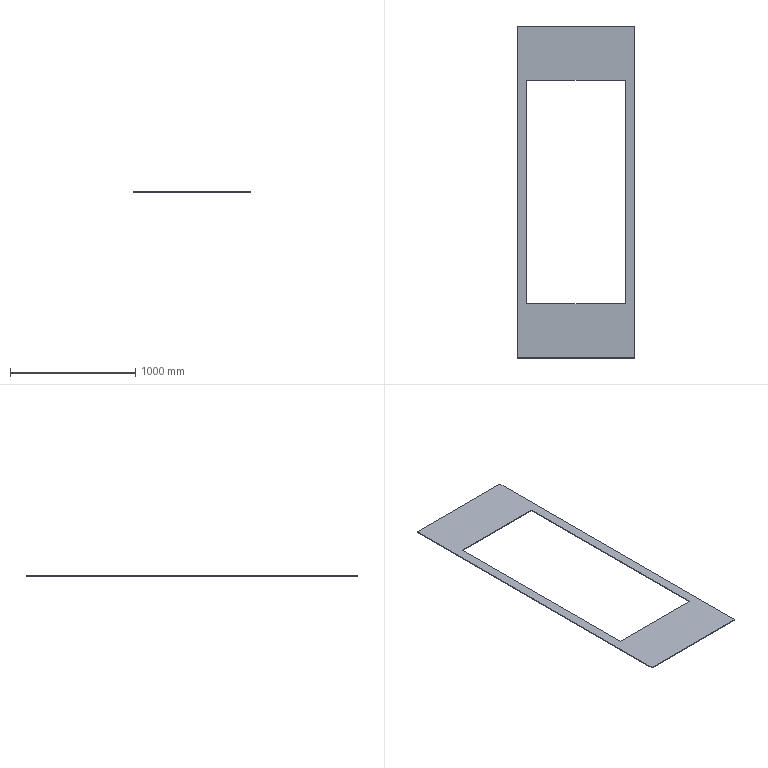Part | STEP file | Bottom plate 6_Default<As machined> | 1 solid | 10 faces | box 934 x 2650 x 6 mm | volume 6458664 mm3 | plane 10
STEP:
#1=CARTESIAN_POINT('',(0.,0.,0.));
#2=DIRECTION('',(0.,0.,1.));
#3=DIRECTION('',(1.,0.,0.));
#4=AXIS2_PLACEMENT_3D('',#1,#2,#3);
#5=CARTESIAN_POINT('',(467.,-1325.,6.));
#6=VERTEX_POINT('',#5);
#7=CARTESIAN_POINT('',(467.,1325.,6.));
#8=VERTEX_POINT('',#7);
#9=CARTESIAN_POINT('',(467.,1325.,6.));
#10=DIRECTION('',(0.,1.,0.));
#11=VECTOR('',#10,1.);
#12=LINE('',#9,#11);
#13=CARTESIAN_POINT('',(0.,0.,6.));
#14=DIRECTION('',(0.,0.,1.));
#15=DIRECTION('',(1.,0.,0.));
#16=AXIS2_PLACEMENT_3D('',#13,#14,#15);
#17=PLANE('',#16);
#18=CARTESIAN_POINT('',(467.,1325.));
#19=DIRECTION('',(0.,1.));
#20=VECTOR('',#19,1.);
#21=LINE('',#18,#20);
#22=(GEOMETRIC_REPRESENTATION_CONTEXT(2)PARAMETRIC_REPRESENTATION_CONTEXT()REPRESENTATION_CONTEXT('',''));
#23=DEFINITIONAL_REPRESENTATION('',(#21),#22);
#24=PCURVE('',#17,#23);
#25=CARTESIAN_POINT('',(467.,1325.,6.));
#26=DIRECTION('',(-1.,0.,0.));
#27=DIRECTION('',(0.,-1.,0.));
#28=AXIS2_PLACEMENT_3D('',#25,#26,#27);
#29=PLANE('',#28);
#30=CARTESIAN_POINT('',(0.,0.));
#31=DIRECTION('',(-1.,0.));
#32=VECTOR('',#31,1.);
#33=LINE('',#30,#32);
#34=(GEOMETRIC_REPRESENTATION_CONTEXT(2)PARAMETRIC_REPRESENTATION_CONTEXT()REPRESENTATION_CONTEXT('',''));
#35=DEFINITIONAL_REPRESENTATION('',(#33),#34);
#36=PCURVE('',#29,#35);
#37=SURFACE_CURVE('',#12,(#24,#36),.PCURVE_S1.);
#38=EDGE_CURVE('',#6,#8,#37,.T.);
#39=ORIENTED_EDGE('',*,*,#38,.T.);
#40=CARTESIAN_POINT('',(-467.,1325.,6.));
#41=VERTEX_POINT('',#40);
#42=CARTESIAN_POINT('',(-467.,1325.,6.));
#43=DIRECTION('',(-1.,0.,0.));
#44=VECTOR('',#43,1.);
#45=LINE('',#42,#44);
#46=CARTESIAN_POINT('',(-467.,1325.));
#47=DIRECTION('',(-1.,0.));
#48=VECTOR('',#47,1.);
#49=LINE('',#46,#48);
#50=(GEOMETRIC_REPRESENTATION_CONTEXT(2)PARAMETRIC_REPRESENTATION_CONTEXT()REPRESENTATION_CONTEXT('',''));
#51=DEFINITIONAL_REPRESENTATION('',(#49),#50);
#52=PCURVE('',#17,#51);
#53=CARTESIAN_POINT('',(-467.,1325.,6.));
#54=DIRECTION('',(0.,-1.,0.));
#55=DIRECTION('',(0.,0.,-1.));
#56=AXIS2_PLACEMENT_3D('',#53,#54,#55);
#57=PLANE('',#56);
#58=CARTESIAN_POINT('',(0.,0.));
#59=DIRECTION('',(0.,-1.));
#60=VECTOR('',#59,1.);
#61=LINE('',#58,#60);
#62=(GEOMETRIC_REPRESENTATION_CONTEXT(2)PARAMETRIC_REPRESENTATION_CONTEXT()REPRESENTATION_CONTEXT('',''));
#63=DEFINITIONAL_REPRESENTATION('',(#61),#62);
#64=PCURVE('',#57,#63);
#65=SURFACE_CURVE('',#45,(#52,#64),.PCURVE_S1.);
#66=EDGE_CURVE('',#8,#41,#65,.T.);
#67=ORIENTED_EDGE('',*,*,#66,.T.);
#68=CARTESIAN_POINT('',(-467.,-1325.,6.));
#69=VERTEX_POINT('',#68);
#70=CARTESIAN_POINT('',(-467.,1325.,6.));
#71=DIRECTION('',(0.,-1.,0.));
#72=VECTOR('',#71,1.);
#73=LINE('',#70,#72);
#74=CARTESIAN_POINT('',(-467.,1325.));
#75=DIRECTION('',(0.,-1.));
#76=VECTOR('',#75,1.);
#77=LINE('',#74,#76);
#78=(GEOMETRIC_REPRESENTATION_CONTEXT(2)PARAMETRIC_REPRESENTATION_CONTEXT()REPRESENTATION_CONTEXT('',''));
#79=DEFINITIONAL_REPRESENTATION('',(#77),#78);
#80=PCURVE('',#17,#79);
#81=CARTESIAN_POINT('',(-467.,1325.,6.));
#82=DIRECTION('',(1.,0.,0.));
#83=DIRECTION('',(0.,1.,0.));
#84=AXIS2_PLACEMENT_3D('',#81,#82,#83);
#85=PLANE('',#84);
#86=CARTESIAN_POINT('',(0.,0.));
#87=DIRECTION('',(-1.,0.));
#88=VECTOR('',#87,1.);
#89=LINE('',#86,#88);
#90=(GEOMETRIC_REPRESENTATION_CONTEXT(2)PARAMETRIC_REPRESENTATION_CONTEXT()REPRESENTATION_CONTEXT('',''));
#91=DEFINITIONAL_REPRESENTATION('',(#89),#90);
#92=PCURVE('',#85,#91);
#93=SURFACE_CURVE('',#73,(#80,#92),.PCURVE_S1.);
#94=EDGE_CURVE('',#41,#69,#93,.T.);
#95=ORIENTED_EDGE('',*,*,#94,.T.);
#96=CARTESIAN_POINT('',(-467.,-1325.,6.));
#97=DIRECTION('',(1.,0.,0.));
#98=VECTOR('',#97,1.);
#99=LINE('',#96,#98);
#100=CARTESIAN_POINT('',(-467.,-1325.));
#101=DIRECTION('',(1.,0.));
#102=VECTOR('',#101,1.);
#103=LINE('',#100,#102);
#104=(GEOMETRIC_REPRESENTATION_CONTEXT(2)PARAMETRIC_REPRESENTATION_CONTEXT()REPRESENTATION_CONTEXT('',''));
#105=DEFINITIONAL_REPRESENTATION('',(#103),#104);
#106=PCURVE('',#17,#105);
#107=CARTESIAN_POINT('',(-467.,-1325.,6.));
#108=DIRECTION('',(0.,1.,0.));
#109=DIRECTION('',(0.,0.,1.));
#110=AXIS2_PLACEMENT_3D('',#107,#108,#109);
#111=PLANE('',#110);
#112=CARTESIAN_POINT('',(0.,0.));
#113=DIRECTION('',(0.,1.));
#114=VECTOR('',#113,1.);
#115=LINE('',#112,#114);
#116=(GEOMETRIC_REPRESENTATION_CONTEXT(2)PARAMETRIC_REPRESENTATION_CONTEXT()REPRESENTATION_CONTEXT('',''));
#117=DEFINITIONAL_REPRESENTATION('',(#115),#116);
#118=PCURVE('',#111,#117);
#119=SURFACE_CURVE('',#99,(#106,#118),.PCURVE_S1.);
#120=EDGE_CURVE('',#69,#6,#119,.T.);
#121=ORIENTED_EDGE('',*,*,#120,.T.);
#122=EDGE_LOOP('',(#39,#67,#95,#121));
#123=FACE_BOUND('',#122,.T.);
#124=CARTESIAN_POINT('',(392.,892.,6.));
#125=VERTEX_POINT('',#124);
#126=CARTESIAN_POINT('',(-392.,892.,6.));
#127=VERTEX_POINT('',#126);
#128=CARTESIAN_POINT('',(-392.,892.,6.));
#129=DIRECTION('',(-1.,0.,0.));
#130=VECTOR('',#129,1.);
#131=LINE('',#128,#130);
#132=CARTESIAN_POINT('',(-392.,892.));
#133=DIRECTION('',(-1.,0.));
#134=VECTOR('',#133,1.);
#135=LINE('',#132,#134);
#136=(GEOMETRIC_REPRESENTATION_CONTEXT(2)PARAMETRIC_REPRESENTATION_CONTEXT()REPRESENTATION_CONTEXT('',''));
#137=DEFINITIONAL_REPRESENTATION('',(#135),#136);
#138=PCURVE('',#17,#137);
#139=CARTESIAN_POINT('',(-392.,892.,6.));
#140=DIRECTION('',(0.,-1.,0.));
#141=DIRECTION('',(0.,0.,-1.));
#142=AXIS2_PLACEMENT_3D('',#139,#140,#141);
#143=PLANE('',#142);
#144=CARTESIAN_POINT('',(0.,0.));
#145=DIRECTION('',(0.,-1.));
#146=VECTOR('',#145,1.);
#147=LINE('',#144,#146);
#148=(GEOMETRIC_REPRESENTATION_CONTEXT(2)PARAMETRIC_REPRESENTATION_CONTEXT()REPRESENTATION_CONTEXT('',''));
#149=DEFINITIONAL_REPRESENTATION('',(#147),#148);
#150=PCURVE('',#143,#149);
#151=SURFACE_CURVE('',#131,(#138,#150),.PCURVE_S1.);
#152=EDGE_CURVE('',#125,#127,#151,.T.);
#153=ORIENTED_EDGE('',*,*,#152,.F.);
#154=CARTESIAN_POINT('',(392.,-892.,6.));
#155=VERTEX_POINT('',#154);
#156=CARTESIAN_POINT('',(392.,892.,6.));
#157=DIRECTION('',(0.,1.,0.));
#158=VECTOR('',#157,1.);
#159=LINE('',#156,#158);
#160=CARTESIAN_POINT('',(392.,892.));
#161=DIRECTION('',(0.,1.));
#162=VECTOR('',#161,1.);
#163=LINE('',#160,#162);
#164=(GEOMETRIC_REPRESENTATION_CONTEXT(2)PARAMETRIC_REPRESENTATION_CONTEXT()REPRESENTATION_CONTEXT('',''));
#165=DEFINITIONAL_REPRESENTATION('',(#163),#164);
#166=PCURVE('',#17,#165);
#167=CARTESIAN_POINT('',(392.,892.,6.));
#168=DIRECTION('',(-1.,0.,0.));
#169=DIRECTION('',(0.,-1.,0.));
#170=AXIS2_PLACEMENT_3D('',#167,#168,#169);
#171=PLANE('',#170);
#172=CARTESIAN_POINT('',(0.,0.));
#173=DIRECTION('',(-1.,0.));
#174=VECTOR('',#173,1.);
#175=LINE('',#172,#174);
#176=(GEOMETRIC_REPRESENTATION_CONTEXT(2)PARAMETRIC_REPRESENTATION_CONTEXT()REPRESENTATION_CONTEXT('',''));
#177=DEFINITIONAL_REPRESENTATION('',(#175),#176);
#178=PCURVE('',#171,#177);
#179=SURFACE_CURVE('',#159,(#166,#178),.PCURVE_S1.);
#180=EDGE_CURVE('',#155,#125,#179,.T.);
#181=ORIENTED_EDGE('',*,*,#180,.F.);
#182=CARTESIAN_POINT('',(-392.,-892.,6.));
#183=VERTEX_POINT('',#182);
#184=CARTESIAN_POINT('',(-392.,-892.,6.));
#185=DIRECTION('',(1.,0.,0.));
#186=VECTOR('',#185,1.);
#187=LINE('',#184,#186);
#188=CARTESIAN_POINT('',(-392.,-892.));
#189=DIRECTION('',(1.,0.));
#190=VECTOR('',#189,1.);
#191=LINE('',#188,#190);
#192=(GEOMETRIC_REPRESENTATION_CONTEXT(2)PARAMETRIC_REPRESENTATION_CONTEXT()REPRESENTATION_CONTEXT('',''));
#193=DEFINITIONAL_REPRESENTATION('',(#191),#192);
#194=PCURVE('',#17,#193);
#195=CARTESIAN_POINT('',(-392.,-892.,6.));
#196=DIRECTION('',(0.,1.,0.));
#197=DIRECTION('',(0.,0.,1.));
#198=AXIS2_PLACEMENT_3D('',#195,#196,#197);
#199=PLANE('',#198);
#200=CARTESIAN_POINT('',(0.,0.));
#201=DIRECTION('',(0.,1.));
#202=VECTOR('',#201,1.);
#203=LINE('',#200,#202);
#204=(GEOMETRIC_REPRESENTATION_CONTEXT(2)PARAMETRIC_REPRESENTATION_CONTEXT()REPRESENTATION_CONTEXT('',''));
#205=DEFINITIONAL_REPRESENTATION('',(#203),#204);
#206=PCURVE('',#199,#205);
#207=SURFACE_CURVE('',#187,(#194,#206),.PCURVE_S1.);
#208=EDGE_CURVE('',#183,#155,#207,.T.);
#209=ORIENTED_EDGE('',*,*,#208,.F.);
#210=CARTESIAN_POINT('',(-392.,892.,6.));
#211=DIRECTION('',(0.,-1.,0.));
#212=VECTOR('',#211,1.);
#213=LINE('',#210,#212);
#214=CARTESIAN_POINT('',(-392.,892.));
#215=DIRECTION('',(0.,-1.));
#216=VECTOR('',#215,1.);
#217=LINE('',#214,#216);
#218=(GEOMETRIC_REPRESENTATION_CONTEXT(2)PARAMETRIC_REPRESENTATION_CONTEXT()REPRESENTATION_CONTEXT('',''));
#219=DEFINITIONAL_REPRESENTATION('',(#217),#218);
#220=PCURVE('',#17,#219);
#221=CARTESIAN_POINT('',(-392.,892.,6.));
#222=DIRECTION('',(1.,0.,0.));
#223=DIRECTION('',(0.,1.,0.));
#224=AXIS2_PLACEMENT_3D('',#221,#222,#223);
#225=PLANE('',#224);
#226=CARTESIAN_POINT('',(0.,0.));
#227=DIRECTION('',(-1.,0.));
#228=VECTOR('',#227,1.);
#229=LINE('',#226,#228);
#230=(GEOMETRIC_REPRESENTATION_CONTEXT(2)PARAMETRIC_REPRESENTATION_CONTEXT()REPRESENTATION_CONTEXT('',''));
#231=DEFINITIONAL_REPRESENTATION('',(#229),#230);
#232=PCURVE('',#225,#231);
#233=SURFACE_CURVE('',#213,(#220,#232),.PCURVE_S1.);
#234=EDGE_CURVE('',#127,#183,#233,.T.);
#235=ORIENTED_EDGE('',*,*,#234,.F.);
#236=EDGE_LOOP('',(#153,#181,#209,#235));
#237=FACE_BOUND('',#236,.T.);
#238=ADVANCED_FACE('',(#123,#237),#17,.T.);
#239=CARTESIAN_POINT('',(467.,-1325.,0.));
#240=VERTEX_POINT('',#239);
#241=CARTESIAN_POINT('',(467.,1325.,0.));
#242=VERTEX_POINT('',#241);
#243=CARTESIAN_POINT('',(467.,1325.,0.));
#244=DIRECTION('',(0.,1.,0.));
#245=VECTOR('',#244,1.);
#246=LINE('',#243,#245);
#247=CARTESIAN_POINT('',(0.,0.,0.));
#248=DIRECTION('',(0.,0.,1.));
#249=DIRECTION('',(1.,0.,0.));
#250=AXIS2_PLACEMENT_3D('',#247,#248,#249);
#251=PLANE('',#250);
#252=CARTESIAN_POINT('',(467.,1325.));
#253=DIRECTION('',(0.,1.));
#254=VECTOR('',#253,1.);
#255=LINE('',#252,#254);
#256=(GEOMETRIC_REPRESENTATION_CONTEXT(2)PARAMETRIC_REPRESENTATION_CONTEXT()REPRESENTATION_CONTEXT('',''));
#257=DEFINITIONAL_REPRESENTATION('',(#255),#256);
#258=PCURVE('',#251,#257);
#259=CARTESIAN_POINT('',(0.,-6.));
#260=DIRECTION('',(-1.,0.));
#261=VECTOR('',#260,1.);
#262=LINE('',#259,#261);
#263=(GEOMETRIC_REPRESENTATION_CONTEXT(2)PARAMETRIC_REPRESENTATION_CONTEXT()REPRESENTATION_CONTEXT('',''));
#264=DEFINITIONAL_REPRESENTATION('',(#262),#263);
#265=PCURVE('',#29,#264);
#266=SURFACE_CURVE('',#246,(#258,#265),.PCURVE_S1.);
#267=EDGE_CURVE('',#240,#242,#266,.T.);
#268=ORIENTED_EDGE('',*,*,#267,.F.);
#269=CARTESIAN_POINT('',(-467.,-1325.,0.));
#270=VERTEX_POINT('',#269);
#271=CARTESIAN_POINT('',(-467.,-1325.,0.));
#272=DIRECTION('',(1.,0.,0.));
#273=VECTOR('',#272,1.);
#274=LINE('',#271,#273);
#275=CARTESIAN_POINT('',(-467.,-1325.));
#276=DIRECTION('',(1.,0.));
#277=VECTOR('',#276,1.);
#278=LINE('',#275,#277);
#279=(GEOMETRIC_REPRESENTATION_CONTEXT(2)PARAMETRIC_REPRESENTATION_CONTEXT()REPRESENTATION_CONTEXT('',''));
#280=DEFINITIONAL_REPRESENTATION('',(#278),#279);
#281=PCURVE('',#251,#280);
#282=CARTESIAN_POINT('',(-6.,0.));
#283=DIRECTION('',(0.,1.));
#284=VECTOR('',#283,1.);
#285=LINE('',#282,#284);
#286=(GEOMETRIC_REPRESENTATION_CONTEXT(2)PARAMETRIC_REPRESENTATION_CONTEXT()REPRESENTATION_CONTEXT('',''));
#287=DEFINITIONAL_REPRESENTATION('',(#285),#286);
#288=PCURVE('',#111,#287);
#289=SURFACE_CURVE('',#274,(#281,#288),.PCURVE_S1.);
#290=EDGE_CURVE('',#270,#240,#289,.T.);
#291=ORIENTED_EDGE('',*,*,#290,.F.);
#292=CARTESIAN_POINT('',(-467.,1325.,0.));
#293=VERTEX_POINT('',#292);
#294=CARTESIAN_POINT('',(-467.,1325.,0.));
#295=DIRECTION('',(0.,-1.,0.));
#296=VECTOR('',#295,1.);
#297=LINE('',#294,#296);
#298=CARTESIAN_POINT('',(-467.,1325.));
#299=DIRECTION('',(0.,-1.));
#300=VECTOR('',#299,1.);
#301=LINE('',#298,#300);
#302=(GEOMETRIC_REPRESENTATION_CONTEXT(2)PARAMETRIC_REPRESENTATION_CONTEXT()REPRESENTATION_CONTEXT('',''));
#303=DEFINITIONAL_REPRESENTATION('',(#301),#302);
#304=PCURVE('',#251,#303);
#305=CARTESIAN_POINT('',(0.,-6.));
#306=DIRECTION('',(-1.,0.));
#307=VECTOR('',#306,1.);
#308=LINE('',#305,#307);
#309=(GEOMETRIC_REPRESENTATION_CONTEXT(2)PARAMETRIC_REPRESENTATION_CONTEXT()REPRESENTATION_CONTEXT('',''));
#310=DEFINITIONAL_REPRESENTATION('',(#308),#309);
#311=PCURVE('',#85,#310);
#312=SURFACE_CURVE('',#297,(#304,#311),.PCURVE_S1.);
#313=EDGE_CURVE('',#293,#270,#312,.T.);
#314=ORIENTED_EDGE('',*,*,#313,.F.);
#315=CARTESIAN_POINT('',(-467.,1325.,0.));
#316=DIRECTION('',(-1.,0.,0.));
#317=VECTOR('',#316,1.);
#318=LINE('',#315,#317);
#319=CARTESIAN_POINT('',(-467.,1325.));
#320=DIRECTION('',(-1.,0.));
#321=VECTOR('',#320,1.);
#322=LINE('',#319,#321);
#323=(GEOMETRIC_REPRESENTATION_CONTEXT(2)PARAMETRIC_REPRESENTATION_CONTEXT()REPRESENTATION_CONTEXT('',''));
#324=DEFINITIONAL_REPRESENTATION('',(#322),#323);
#325=PCURVE('',#251,#324);
#326=CARTESIAN_POINT('',(6.,0.));
#327=DIRECTION('',(0.,-1.));
#328=VECTOR('',#327,1.);
#329=LINE('',#326,#328);
#330=(GEOMETRIC_REPRESENTATION_CONTEXT(2)PARAMETRIC_REPRESENTATION_CONTEXT()REPRESENTATION_CONTEXT('',''));
#331=DEFINITIONAL_REPRESENTATION('',(#329),#330);
#332=PCURVE('',#57,#331);
#333=SURFACE_CURVE('',#318,(#325,#332),.PCURVE_S1.);
#334=EDGE_CURVE('',#242,#293,#333,.T.);
#335=ORIENTED_EDGE('',*,*,#334,.F.);
#336=EDGE_LOOP('',(#268,#291,#314,#335));
#337=FACE_BOUND('',#336,.T.);
#338=CARTESIAN_POINT('',(392.,-892.,0.));
#339=VERTEX_POINT('',#338);
#340=CARTESIAN_POINT('',(392.,892.,0.));
#341=VERTEX_POINT('',#340);
#342=CARTESIAN_POINT('',(392.,892.,0.));
#343=DIRECTION('',(0.,1.,0.));
#344=VECTOR('',#343,1.);
#345=LINE('',#342,#344);
#346=CARTESIAN_POINT('',(392.,892.));
#347=DIRECTION('',(0.,1.));
#348=VECTOR('',#347,1.);
#349=LINE('',#346,#348);
#350=(GEOMETRIC_REPRESENTATION_CONTEXT(2)PARAMETRIC_REPRESENTATION_CONTEXT()REPRESENTATION_CONTEXT('',''));
#351=DEFINITIONAL_REPRESENTATION('',(#349),#350);
#352=PCURVE('',#251,#351);
#353=CARTESIAN_POINT('',(0.,-6.));
#354=DIRECTION('',(-1.,0.));
#355=VECTOR('',#354,1.);
#356=LINE('',#353,#355);
#357=(GEOMETRIC_REPRESENTATION_CONTEXT(2)PARAMETRIC_REPRESENTATION_CONTEXT()REPRESENTATION_CONTEXT('',''));
#358=DEFINITIONAL_REPRESENTATION('',(#356),#357);
#359=PCURVE('',#171,#358);
#360=SURFACE_CURVE('',#345,(#352,#359),.PCURVE_S1.);
#361=EDGE_CURVE('',#339,#341,#360,.T.);
#362=ORIENTED_EDGE('',*,*,#361,.T.);
#363=CARTESIAN_POINT('',(-392.,892.,0.));
#364=VERTEX_POINT('',#363);
#365=CARTESIAN_POINT('',(-392.,892.,0.));
#366=DIRECTION('',(-1.,0.,0.));
#367=VECTOR('',#366,1.);
#368=LINE('',#365,#367);
#369=CARTESIAN_POINT('',(-392.,892.));
#370=DIRECTION('',(-1.,0.));
#371=VECTOR('',#370,1.);
#372=LINE('',#369,#371);
#373=(GEOMETRIC_REPRESENTATION_CONTEXT(2)PARAMETRIC_REPRESENTATION_CONTEXT()REPRESENTATION_CONTEXT('',''));
#374=DEFINITIONAL_REPRESENTATION('',(#372),#373);
#375=PCURVE('',#251,#374);
#376=CARTESIAN_POINT('',(6.,0.));
#377=DIRECTION('',(0.,-1.));
#378=VECTOR('',#377,1.);
#379=LINE('',#376,#378);
#380=(GEOMETRIC_REPRESENTATION_CONTEXT(2)PARAMETRIC_REPRESENTATION_CONTEXT()REPRESENTATION_CONTEXT('',''));
#381=DEFINITIONAL_REPRESENTATION('',(#379),#380);
#382=PCURVE('',#143,#381);
#383=SURFACE_CURVE('',#368,(#375,#382),.PCURVE_S1.);
#384=EDGE_CURVE('',#341,#364,#383,.T.);
#385=ORIENTED_EDGE('',*,*,#384,.T.);
#386=CARTESIAN_POINT('',(-392.,-892.,0.));
#387=VERTEX_POINT('',#386);
#388=CARTESIAN_POINT('',(-392.,892.,0.));
#389=DIRECTION('',(0.,-1.,0.));
#390=VECTOR('',#389,1.);
#391=LINE('',#388,#390);
#392=CARTESIAN_POINT('',(-392.,892.));
#393=DIRECTION('',(0.,-1.));
#394=VECTOR('',#393,1.);
#395=LINE('',#392,#394);
#396=(GEOMETRIC_REPRESENTATION_CONTEXT(2)PARAMETRIC_REPRESENTATION_CONTEXT()REPRESENTATION_CONTEXT('',''));
#397=DEFINITIONAL_REPRESENTATION('',(#395),#396);
#398=PCURVE('',#251,#397);
#399=CARTESIAN_POINT('',(0.,-6.));
#400=DIRECTION('',(-1.,0.));
#401=VECTOR('',#400,1.);
#402=LINE('',#399,#401);
#403=(GEOMETRIC_REPRESENTATION_CONTEXT(2)PARAMETRIC_REPRESENTATION_CONTEXT()REPRESENTATION_CONTEXT('',''));
#404=DEFINITIONAL_REPRESENTATION('',(#402),#403);
#405=PCURVE('',#225,#404);
#406=SURFACE_CURVE('',#391,(#398,#405),.PCURVE_S1.);
#407=EDGE_CURVE('',#364,#387,#406,.T.);
#408=ORIENTED_EDGE('',*,*,#407,.T.);
#409=CARTESIAN_POINT('',(-392.,-892.,0.));
#410=DIRECTION('',(1.,0.,0.));
#411=VECTOR('',#410,1.);
#412=LINE('',#409,#411);
#413=CARTESIAN_POINT('',(-392.,-892.));
#414=DIRECTION('',(1.,0.));
#415=VECTOR('',#414,1.);
#416=LINE('',#413,#415);
#417=(GEOMETRIC_REPRESENTATION_CONTEXT(2)PARAMETRIC_REPRESENTATION_CONTEXT()REPRESENTATION_CONTEXT('',''));
#418=DEFINITIONAL_REPRESENTATION('',(#416),#417);
#419=PCURVE('',#251,#418);
#420=CARTESIAN_POINT('',(-6.,0.));
#421=DIRECTION('',(0.,1.));
#422=VECTOR('',#421,1.);
#423=LINE('',#420,#422);
#424=(GEOMETRIC_REPRESENTATION_CONTEXT(2)PARAMETRIC_REPRESENTATION_CONTEXT()REPRESENTATION_CONTEXT('',''));
#425=DEFINITIONAL_REPRESENTATION('',(#423),#424);
#426=PCURVE('',#199,#425);
#427=SURFACE_CURVE('',#412,(#419,#426),.PCURVE_S1.);
#428=EDGE_CURVE('',#387,#339,#427,.T.);
#429=ORIENTED_EDGE('',*,*,#428,.T.);
#430=EDGE_LOOP('',(#362,#385,#408,#429));
#431=FACE_BOUND('',#430,.T.);
#432=ADVANCED_FACE('',(#337,#431),#251,.F.);
#433=ORIENTED_EDGE('',*,*,#267,.T.);
#434=CARTESIAN_POINT('',(467.,1325.,6.));
#435=DIRECTION('',(0.,0.,-1.));
#436=VECTOR('',#435,1.);
#437=LINE('',#434,#436);
#438=CARTESIAN_POINT('',(0.,0.));
#439=DIRECTION('',(0.,-1.));
#440=VECTOR('',#439,1.);
#441=LINE('',#438,#440);
#442=(GEOMETRIC_REPRESENTATION_CONTEXT(2)PARAMETRIC_REPRESENTATION_CONTEXT()REPRESENTATION_CONTEXT('',''));
#443=DEFINITIONAL_REPRESENTATION('',(#441),#442);
#444=PCURVE('',#29,#443);
#445=CARTESIAN_POINT('',(0.,934.));
#446=DIRECTION('',(1.,0.));
#447=VECTOR('',#446,1.);
#448=LINE('',#445,#447);
#449=(GEOMETRIC_REPRESENTATION_CONTEXT(2)PARAMETRIC_REPRESENTATION_CONTEXT()REPRESENTATION_CONTEXT('',''));
#450=DEFINITIONAL_REPRESENTATION('',(#448),#449);
#451=PCURVE('',#57,#450);
#452=SURFACE_CURVE('',#437,(#444,#451),.PCURVE_S1.);
#453=EDGE_CURVE('',#8,#242,#452,.T.);
#454=ORIENTED_EDGE('',*,*,#453,.F.);
#455=ORIENTED_EDGE('',*,*,#38,.F.);
#456=CARTESIAN_POINT('',(467.,-1325.,6.));
#457=DIRECTION('',(0.,0.,-1.));
#458=VECTOR('',#457,1.);
#459=LINE('',#456,#458);
#460=CARTESIAN_POINT('',(2650.,0.));
#461=DIRECTION('',(0.,-1.));
#462=VECTOR('',#461,1.);
#463=LINE('',#460,#462);
#464=(GEOMETRIC_REPRESENTATION_CONTEXT(2)PARAMETRIC_REPRESENTATION_CONTEXT()REPRESENTATION_CONTEXT('',''));
#465=DEFINITIONAL_REPRESENTATION('',(#463),#464);
#466=PCURVE('',#29,#465);
#467=CARTESIAN_POINT('',(0.,934.));
#468=DIRECTION('',(-1.,0.));
#469=VECTOR('',#468,1.);
#470=LINE('',#467,#469);
#471=(GEOMETRIC_REPRESENTATION_CONTEXT(2)PARAMETRIC_REPRESENTATION_CONTEXT()REPRESENTATION_CONTEXT('',''));
#472=DEFINITIONAL_REPRESENTATION('',(#470),#471);
#473=PCURVE('',#111,#472);
#474=SURFACE_CURVE('',#459,(#466,#473),.PCURVE_S1.);
#475=EDGE_CURVE('',#6,#240,#474,.T.);
#476=ORIENTED_EDGE('',*,*,#475,.T.);
#477=EDGE_LOOP('',(#433,#454,#455,#476));
#478=FACE_BOUND('',#477,.T.);
#479=ADVANCED_FACE('',(#478),#29,.F.);
#480=ORIENTED_EDGE('',*,*,#334,.T.);
#481=CARTESIAN_POINT('',(-467.,1325.,6.));
#482=DIRECTION('',(0.,0.,-1.));
#483=VECTOR('',#482,1.);
#484=LINE('',#481,#483);
#485=CARTESIAN_POINT('',(0.,0.));
#486=DIRECTION('',(1.,0.));
#487=VECTOR('',#486,1.);
#488=LINE('',#485,#487);
#489=(GEOMETRIC_REPRESENTATION_CONTEXT(2)PARAMETRIC_REPRESENTATION_CONTEXT()REPRESENTATION_CONTEXT('',''));
#490=DEFINITIONAL_REPRESENTATION('',(#488),#489);
#491=PCURVE('',#57,#490);
#492=CARTESIAN_POINT('',(0.,0.));
#493=DIRECTION('',(0.,-1.));
#494=VECTOR('',#493,1.);
#495=LINE('',#492,#494);
#496=(GEOMETRIC_REPRESENTATION_CONTEXT(2)PARAMETRIC_REPRESENTATION_CONTEXT()REPRESENTATION_CONTEXT('',''));
#497=DEFINITIONAL_REPRESENTATION('',(#495),#496);
#498=PCURVE('',#85,#497);
#499=SURFACE_CURVE('',#484,(#491,#498),.PCURVE_S1.);
#500=EDGE_CURVE('',#41,#293,#499,.T.);
#501=ORIENTED_EDGE('',*,*,#500,.F.);
#502=ORIENTED_EDGE('',*,*,#66,.F.);
#503=ORIENTED_EDGE('',*,*,#453,.T.);
#504=EDGE_LOOP('',(#480,#501,#502,#503));
#505=FACE_BOUND('',#504,.T.);
#506=ADVANCED_FACE('',(#505),#57,.F.);
#507=ORIENTED_EDGE('',*,*,#313,.T.);
#508=CARTESIAN_POINT('',(-467.,-1325.,6.));
#509=DIRECTION('',(0.,0.,-1.));
#510=VECTOR('',#509,1.);
#511=LINE('',#508,#510);
#512=CARTESIAN_POINT('',(-2650.,0.));
#513=DIRECTION('',(0.,-1.));
#514=VECTOR('',#513,1.);
#515=LINE('',#512,#514);
#516=(GEOMETRIC_REPRESENTATION_CONTEXT(2)PARAMETRIC_REPRESENTATION_CONTEXT()REPRESENTATION_CONTEXT('',''));
#517=DEFINITIONAL_REPRESENTATION('',(#515),#516);
#518=PCURVE('',#85,#517);
#519=CARTESIAN_POINT('',(0.,0.));
#520=DIRECTION('',(-1.,0.));
#521=VECTOR('',#520,1.);
#522=LINE('',#519,#521);
#523=(GEOMETRIC_REPRESENTATION_CONTEXT(2)PARAMETRIC_REPRESENTATION_CONTEXT()REPRESENTATION_CONTEXT('',''));
#524=DEFINITIONAL_REPRESENTATION('',(#522),#523);
#525=PCURVE('',#111,#524);
#526=SURFACE_CURVE('',#511,(#518,#525),.PCURVE_S1.);
#527=EDGE_CURVE('',#69,#270,#526,.T.);
#528=ORIENTED_EDGE('',*,*,#527,.F.);
#529=ORIENTED_EDGE('',*,*,#94,.F.);
#530=ORIENTED_EDGE('',*,*,#500,.T.);
#531=EDGE_LOOP('',(#507,#528,#529,#530));
#532=FACE_BOUND('',#531,.T.);
#533=ADVANCED_FACE('',(#532),#85,.F.);
#534=ORIENTED_EDGE('',*,*,#290,.T.);
#535=ORIENTED_EDGE('',*,*,#475,.F.);
#536=ORIENTED_EDGE('',*,*,#120,.F.);
#537=ORIENTED_EDGE('',*,*,#527,.T.);
#538=EDGE_LOOP('',(#534,#535,#536,#537));
#539=FACE_BOUND('',#538,.T.);
#540=ADVANCED_FACE('',(#539),#111,.F.);
#541=ORIENTED_EDGE('',*,*,#361,.F.);
#542=CARTESIAN_POINT('',(392.,-892.,6.));
#543=DIRECTION('',(0.,0.,-1.));
#544=VECTOR('',#543,1.);
#545=LINE('',#542,#544);
#546=CARTESIAN_POINT('',(1784.,0.));
#547=DIRECTION('',(0.,-1.));
#548=VECTOR('',#547,1.);
#549=LINE('',#546,#548);
#550=(GEOMETRIC_REPRESENTATION_CONTEXT(2)PARAMETRIC_REPRESENTATION_CONTEXT()REPRESENTATION_CONTEXT('',''));
#551=DEFINITIONAL_REPRESENTATION('',(#549),#550);
#552=PCURVE('',#171,#551);
#553=CARTESIAN_POINT('',(0.,784.));
#554=DIRECTION('',(-1.,0.));
#555=VECTOR('',#554,1.);
#556=LINE('',#553,#555);
#557=(GEOMETRIC_REPRESENTATION_CONTEXT(2)PARAMETRIC_REPRESENTATION_CONTEXT()REPRESENTATION_CONTEXT('',''));
#558=DEFINITIONAL_REPRESENTATION('',(#556),#557);
#559=PCURVE('',#199,#558);
#560=SURFACE_CURVE('',#545,(#552,#559),.PCURVE_S1.);
#561=EDGE_CURVE('',#155,#339,#560,.T.);
#562=ORIENTED_EDGE('',*,*,#561,.F.);
#563=ORIENTED_EDGE('',*,*,#180,.T.);
#564=CARTESIAN_POINT('',(392.,892.,6.));
#565=DIRECTION('',(0.,0.,-1.));
#566=VECTOR('',#565,1.);
#567=LINE('',#564,#566);
#568=CARTESIAN_POINT('',(0.,0.));
#569=DIRECTION('',(0.,-1.));
#570=VECTOR('',#569,1.);
#571=LINE('',#568,#570);
#572=(GEOMETRIC_REPRESENTATION_CONTEXT(2)PARAMETRIC_REPRESENTATION_CONTEXT()REPRESENTATION_CONTEXT('',''));
#573=DEFINITIONAL_REPRESENTATION('',(#571),#572);
#574=PCURVE('',#171,#573);
#575=CARTESIAN_POINT('',(0.,784.));
#576=DIRECTION('',(1.,0.));
#577=VECTOR('',#576,1.);
#578=LINE('',#575,#577);
#579=(GEOMETRIC_REPRESENTATION_CONTEXT(2)PARAMETRIC_REPRESENTATION_CONTEXT()REPRESENTATION_CONTEXT('',''));
#580=DEFINITIONAL_REPRESENTATION('',(#578),#579);
#581=PCURVE('',#143,#580);
#582=SURFACE_CURVE('',#567,(#574,#581),.PCURVE_S1.);
#583=EDGE_CURVE('',#125,#341,#582,.T.);
#584=ORIENTED_EDGE('',*,*,#583,.T.);
#585=EDGE_LOOP('',(#541,#562,#563,#584));
#586=FACE_BOUND('',#585,.T.);
#587=ADVANCED_FACE('',(#586),#171,.T.);
#588=ORIENTED_EDGE('',*,*,#384,.F.);
#589=ORIENTED_EDGE('',*,*,#583,.F.);
#590=ORIENTED_EDGE('',*,*,#152,.T.);
#591=CARTESIAN_POINT('',(-392.,892.,6.));
#592=DIRECTION('',(0.,0.,-1.));
#593=VECTOR('',#592,1.);
#594=LINE('',#591,#593);
#595=CARTESIAN_POINT('',(0.,0.));
#596=DIRECTION('',(1.,0.));
#597=VECTOR('',#596,1.);
#598=LINE('',#595,#597);
#599=(GEOMETRIC_REPRESENTATION_CONTEXT(2)PARAMETRIC_REPRESENTATION_CONTEXT()REPRESENTATION_CONTEXT('',''));
#600=DEFINITIONAL_REPRESENTATION('',(#598),#599);
#601=PCURVE('',#143,#600);
#602=CARTESIAN_POINT('',(0.,0.));
#603=DIRECTION('',(0.,-1.));
#604=VECTOR('',#603,1.);
#605=LINE('',#602,#604);
#606=(GEOMETRIC_REPRESENTATION_CONTEXT(2)PARAMETRIC_REPRESENTATION_CONTEXT()REPRESENTATION_CONTEXT('',''));
#607=DEFINITIONAL_REPRESENTATION('',(#605),#606);
#608=PCURVE('',#225,#607);
#609=SURFACE_CURVE('',#594,(#601,#608),.PCURVE_S1.);
#610=EDGE_CURVE('',#127,#364,#609,.T.);
#611=ORIENTED_EDGE('',*,*,#610,.T.);
#612=EDGE_LOOP('',(#588,#589,#590,#611));
#613=FACE_BOUND('',#612,.T.);
#614=ADVANCED_FACE('',(#613),#143,.T.);
#615=ORIENTED_EDGE('',*,*,#407,.F.);
#616=ORIENTED_EDGE('',*,*,#610,.F.);
#617=ORIENTED_EDGE('',*,*,#234,.T.);
#618=CARTESIAN_POINT('',(-392.,-892.,6.));
#619=DIRECTION('',(0.,0.,-1.));
#620=VECTOR('',#619,1.);
#621=LINE('',#618,#620);
#622=CARTESIAN_POINT('',(-1784.,0.));
#623=DIRECTION('',(0.,-1.));
#624=VECTOR('',#623,1.);
#625=LINE('',#622,#624);
#626=(GEOMETRIC_REPRESENTATION_CONTEXT(2)PARAMETRIC_REPRESENTATION_CONTEXT()REPRESENTATION_CONTEXT('',''));
#627=DEFINITIONAL_REPRESENTATION('',(#625),#626);
#628=PCURVE('',#225,#627);
#629=CARTESIAN_POINT('',(0.,0.));
#630=DIRECTION('',(-1.,0.));
#631=VECTOR('',#630,1.);
#632=LINE('',#629,#631);
#633=(GEOMETRIC_REPRESENTATION_CONTEXT(2)PARAMETRIC_REPRESENTATION_CONTEXT()REPRESENTATION_CONTEXT('',''));
#634=DEFINITIONAL_REPRESENTATION('',(#632),#633);
#635=PCURVE('',#199,#634);
#636=SURFACE_CURVE('',#621,(#628,#635),.PCURVE_S1.);
#637=EDGE_CURVE('',#183,#387,#636,.T.);
#638=ORIENTED_EDGE('',*,*,#637,.T.);
#639=EDGE_LOOP('',(#615,#616,#617,#638));
#640=FACE_BOUND('',#639,.T.);
#641=ADVANCED_FACE('',(#640),#225,.T.);
#642=ORIENTED_EDGE('',*,*,#428,.F.);
#643=ORIENTED_EDGE('',*,*,#637,.F.);
#644=ORIENTED_EDGE('',*,*,#208,.T.);
#645=ORIENTED_EDGE('',*,*,#561,.T.);
#646=EDGE_LOOP('',(#642,#643,#644,#645));
#647=FACE_BOUND('',#646,.T.);
#648=ADVANCED_FACE('',(#647),#199,.T.);
#649=CLOSED_SHELL('',(#238,#432,#479,#506,#533,#540,#587,#614,#641,#648));
#650=MANIFOLD_SOLID_BREP('',#649);
#651=(LENGTH_UNIT()NAMED_UNIT(*)SI_UNIT(.MILLI.,.METRE.));
#652=UNCERTAINTY_MEASURE_WITH_UNIT(LENGTH_MEASURE(0.0000001),#651,'','');
#653=(NAMED_UNIT(*)PLANE_ANGLE_UNIT()SI_UNIT($,.RADIAN.));
#654=(NAMED_UNIT(*)SI_UNIT($,.STERADIAN.)SOLID_ANGLE_UNIT());
#655=(GEOMETRIC_REPRESENTATION_CONTEXT(3)GLOBAL_UNCERTAINTY_ASSIGNED_CONTEXT((#652))GLOBAL_UNIT_ASSIGNED_CONTEXT((#651,#653,#654))REPRESENTATION_CONTEXT('',''));
#656=ADVANCED_BREP_SHAPE_REPRESENTATION('',(#4,#650),#655);